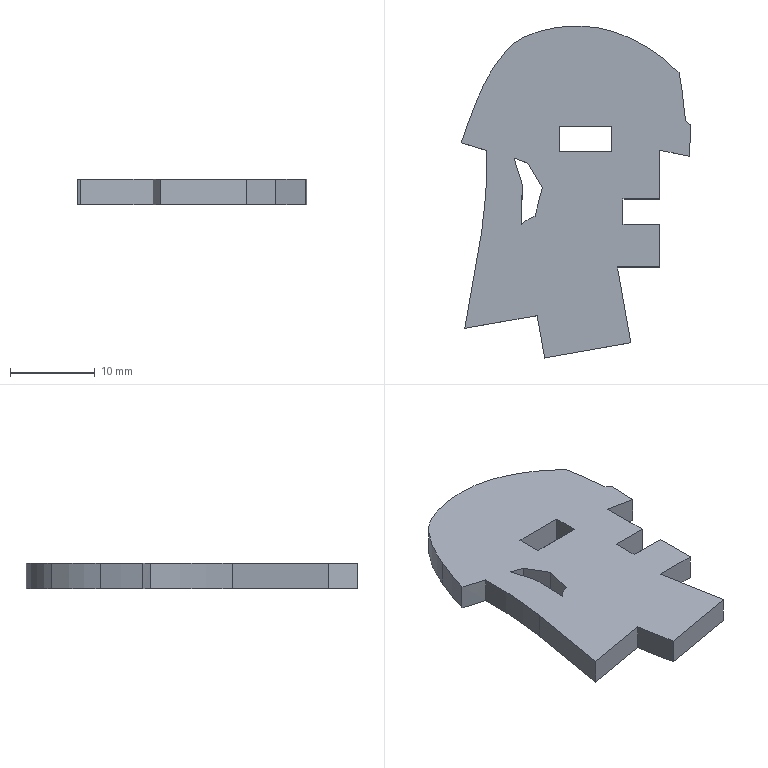Part | SolidWorks | features BaseBody 1 | 1 solid | 33 faces | box 27.077 x 39.16 x 3 mm | volume 2127 mm3 | plane 20 | spline 13
STEP:
#1=CARTESIAN_POINT('',(-12.743,15.285,-1.5));
#2=VERTEX_POINT('',#1);
#3=CARTESIAN_POINT('',(-6.608,15.285,-1.5));
#4=VERTEX_POINT('',#3);
#5=CARTESIAN_POINT('',(-12.743,15.285,-1.5));
#6=DIRECTION('',(1.,0.,0.));
#7=VECTOR('',#6,1000.);
#8=LINE('',#5,#7);
#9=EDGE_CURVE('',#2,#4,#8,.T.);
#10=ORIENTED_EDGE('',*,*,#9,.F.);
#11=CARTESIAN_POINT('',(-12.743,15.285,1.5));
#12=VERTEX_POINT('',#11);
#13=CARTESIAN_POINT('',(-12.743,15.285,1.5));
#14=DIRECTION('',(0.,0.,-1.));
#15=VECTOR('',#14,1000.);
#16=LINE('',#13,#15);
#17=EDGE_CURVE('',#12,#2,#16,.T.);
#18=ORIENTED_EDGE('',*,*,#17,.F.);
#19=CARTESIAN_POINT('',(-6.608,15.285,1.5));
#20=VERTEX_POINT('',#19);
#21=CARTESIAN_POINT('',(-12.743,15.285,1.5));
#22=DIRECTION('',(1.,0.,0.));
#23=VECTOR('',#22,1000.);
#24=LINE('',#21,#23);
#25=EDGE_CURVE('',#12,#20,#24,.T.);
#26=ORIENTED_EDGE('',*,*,#25,.T.);
#27=CARTESIAN_POINT('',(-6.608,15.285,1.5));
#28=DIRECTION('',(0.,0.,-1.));
#29=VECTOR('',#28,1000.);
#30=LINE('',#27,#29);
#31=EDGE_CURVE('',#20,#4,#30,.T.);
#32=ORIENTED_EDGE('',*,*,#31,.T.);
#33=EDGE_LOOP('',(#10,#18,#26,#32));
#34=FACE_OUTER_BOUND('',#33,.T.);
#35=CARTESIAN_POINT('',(-12.743,15.285,1.5));
#36=DIRECTION('',(0.,1.,0.));
#37=DIRECTION('',(1.,0.,0.));
#38=AXIS2_PLACEMENT_3D('',#35,#36,#37);
#39=PLANE('',#38);
#40=ADVANCED_FACE('',(#34),#39,.T.);
#41=CARTESIAN_POINT('',(-12.743,18.281,-1.5));
#42=VERTEX_POINT('',#41);
#43=CARTESIAN_POINT('',(-12.743,18.281,-1.5));
#44=DIRECTION('',(0.,-1.,0.));
#45=VECTOR('',#44,1000.);
#46=LINE('',#43,#45);
#47=EDGE_CURVE('',#42,#2,#46,.T.);
#48=ORIENTED_EDGE('',*,*,#47,.F.);
#49=CARTESIAN_POINT('',(-12.743,18.281,1.5));
#50=VERTEX_POINT('',#49);
#51=CARTESIAN_POINT('',(-12.743,18.281,1.5));
#52=DIRECTION('',(0.,0.,-1.));
#53=VECTOR('',#52,1000.);
#54=LINE('',#51,#53);
#55=EDGE_CURVE('',#50,#42,#54,.T.);
#56=ORIENTED_EDGE('',*,*,#55,.F.);
#57=CARTESIAN_POINT('',(-12.743,18.281,1.5));
#58=DIRECTION('',(0.,-1.,0.));
#59=VECTOR('',#58,1000.);
#60=LINE('',#57,#59);
#61=EDGE_CURVE('',#50,#12,#60,.T.);
#62=ORIENTED_EDGE('',*,*,#61,.T.);
#63=ORIENTED_EDGE('',*,*,#17,.T.);
#64=EDGE_LOOP('',(#48,#56,#62,#63));
#65=FACE_OUTER_BOUND('',#64,.T.);
#66=CARTESIAN_POINT('',(-12.743,18.281,1.5));
#67=DIRECTION('',(1.,0.,0.));
#68=DIRECTION('',(0.,1.,0.));
#69=AXIS2_PLACEMENT_3D('',#66,#67,#68);
#70=PLANE('',#69);
#71=ADVANCED_FACE('',(#65),#70,.T.);
#72=CARTESIAN_POINT('',(-6.608,18.281,-1.5));
#73=VERTEX_POINT('',#72);
#74=CARTESIAN_POINT('',(-6.608,18.281,-1.5));
#75=DIRECTION('',(-1.,0.,0.));
#76=VECTOR('',#75,1000.);
#77=LINE('',#74,#76);
#78=EDGE_CURVE('',#73,#42,#77,.T.);
#79=ORIENTED_EDGE('',*,*,#78,.F.);
#80=CARTESIAN_POINT('',(-6.608,18.281,1.5));
#81=VERTEX_POINT('',#80);
#82=CARTESIAN_POINT('',(-6.608,18.281,1.5));
#83=DIRECTION('',(0.,0.,-1.));
#84=VECTOR('',#83,1000.);
#85=LINE('',#82,#84);
#86=EDGE_CURVE('',#81,#73,#85,.T.);
#87=ORIENTED_EDGE('',*,*,#86,.F.);
#88=CARTESIAN_POINT('',(-6.608,18.281,1.5));
#89=DIRECTION('',(-1.,0.,0.));
#90=VECTOR('',#89,1000.);
#91=LINE('',#88,#90);
#92=EDGE_CURVE('',#81,#50,#91,.T.);
#93=ORIENTED_EDGE('',*,*,#92,.T.);
#94=ORIENTED_EDGE('',*,*,#55,.T.);
#95=EDGE_LOOP('',(#79,#87,#93,#94));
#96=FACE_OUTER_BOUND('',#95,.T.);
#97=CARTESIAN_POINT('',(-6.608,18.281,1.5));
#98=DIRECTION('',(0.,-1.,0.));
#99=DIRECTION('',(0.,0.,-1.));
#100=AXIS2_PLACEMENT_3D('',#97,#98,#99);
#101=PLANE('',#100);
#102=ADVANCED_FACE('',(#96),#101,.T.);
#103=CARTESIAN_POINT('',(-6.608,15.285,-1.5));
#104=DIRECTION('',(0.,1.,0.));
#105=VECTOR('',#104,1000.);
#106=LINE('',#103,#105);
#107=EDGE_CURVE('',#4,#73,#106,.T.);
#108=ORIENTED_EDGE('',*,*,#107,.F.);
#109=ORIENTED_EDGE('',*,*,#31,.F.);
#110=CARTESIAN_POINT('',(-6.608,15.285,1.5));
#111=DIRECTION('',(0.,1.,0.));
#112=VECTOR('',#111,1000.);
#113=LINE('',#110,#112);
#114=EDGE_CURVE('',#20,#81,#113,.T.);
#115=ORIENTED_EDGE('',*,*,#114,.T.);
#116=ORIENTED_EDGE('',*,*,#86,.T.);
#117=EDGE_LOOP('',(#108,#109,#115,#116));
#118=FACE_OUTER_BOUND('',#117,.T.);
#119=CARTESIAN_POINT('',(-6.608,15.285,1.5));
#120=DIRECTION('',(-1.,0.,0.));
#121=DIRECTION('',(0.,1.,0.));
#122=AXIS2_PLACEMENT_3D('',#119,#120,#121);
#123=PLANE('',#122);
#124=ADVANCED_FACE('',(#118),#123,.T.);
#125=CARTESIAN_POINT('',(-16.5,13.932,-1.5));
#126=VERTEX_POINT('',#125);
#127=CARTESIAN_POINT('',(-18.124,14.526,-1.5));
#128=VERTEX_POINT('',#127);
#129=CARTESIAN_POINT('',(-16.5,13.932,-1.5));
#130=CARTESIAN_POINT('',(-17.041,14.129,-1.5));
#131=CARTESIAN_POINT('',(-17.583,14.328,-1.5));
#132=CARTESIAN_POINT('',(-18.124,14.526,-1.5));
#133=B_SPLINE_CURVE_WITH_KNOTS('',3,(#129,#130,#131,#132),.UNSPECIFIED.,.F.,.F.,(4,4),(0.,0.1429),.UNSPECIFIED.);
#134=EDGE_CURVE('',#126,#128,#133,.T.);
#135=ORIENTED_EDGE('',*,*,#134,.F.);
#136=CARTESIAN_POINT('',(-16.5,13.932,1.5));
#137=VERTEX_POINT('',#136);
#138=CARTESIAN_POINT('',(-16.5,13.932,1.5));
#139=DIRECTION('',(0.,0.,-1.));
#140=VECTOR('',#139,1000.);
#141=LINE('',#138,#140);
#142=EDGE_CURVE('',#137,#126,#141,.T.);
#143=ORIENTED_EDGE('',*,*,#142,.F.);
#144=CARTESIAN_POINT('',(-18.124,14.526,1.5));
#145=VERTEX_POINT('',#144);
#146=CARTESIAN_POINT('',(-16.5,13.932,1.5));
#147=CARTESIAN_POINT('',(-17.041,14.129,1.5));
#148=CARTESIAN_POINT('',(-17.583,14.328,1.5));
#149=CARTESIAN_POINT('',(-18.124,14.526,1.5));
#150=B_SPLINE_CURVE_WITH_KNOTS('',3,(#146,#147,#148,#149),.UNSPECIFIED.,.F.,.F.,(4,4),(0.,0.1429),.UNSPECIFIED.);
#151=EDGE_CURVE('',#137,#145,#150,.T.);
#152=ORIENTED_EDGE('',*,*,#151,.T.);
#153=CARTESIAN_POINT('',(-18.124,14.526,1.5));
#154=DIRECTION('',(0.,0.,-1.));
#155=VECTOR('',#154,1000.);
#156=LINE('',#153,#155);
#157=EDGE_CURVE('',#145,#128,#156,.T.);
#158=ORIENTED_EDGE('',*,*,#157,.T.);
#159=EDGE_LOOP('',(#135,#143,#152,#158));
#160=FACE_OUTER_BOUND('',#159,.T.);
#161=CARTESIAN_POINT('',(-16.5,13.932,1.5));
#162=CARTESIAN_POINT('',(-16.5,13.932,-1.5));
#163=CARTESIAN_POINT('',(-17.041,14.129,1.5));
#164=CARTESIAN_POINT('',(-17.041,14.129,-1.5));
#165=CARTESIAN_POINT('',(-17.583,14.328,1.5));
#166=CARTESIAN_POINT('',(-17.583,14.328,-1.5));
#167=CARTESIAN_POINT('',(-18.124,14.526,1.5));
#168=CARTESIAN_POINT('',(-18.124,14.526,-1.5));
#169=B_SPLINE_SURFACE_WITH_KNOTS('',3,1,((#161,#162),(#163,#164),(#165,#166),(#167,#168)),.UNSPECIFIED.,.F.,.F.,.F.,(4,4),(2,2),(0.,0.1429),(0.,1.),.UNSPECIFIED.);
#170=ADVANCED_FACE('',(#160),#169,.T.);
#171=CARTESIAN_POINT('',(-14.796,11.064,-1.5));
#172=VERTEX_POINT('',#171);
#173=CARTESIAN_POINT('',(-14.796,11.064,-1.5));
#174=CARTESIAN_POINT('',(-15.362,12.021,-1.5));
#175=CARTESIAN_POINT('',(-15.932,12.975,-1.5));
#176=CARTESIAN_POINT('',(-16.5,13.932,-1.5));
#177=B_SPLINE_CURVE_WITH_KNOTS('',3,(#173,#174,#175,#176),.UNSPECIFIED.,.F.,.F.,(4,4),(0.1429,0.2857),.UNSPECIFIED.);
#178=EDGE_CURVE('',#172,#126,#177,.T.);
#179=ORIENTED_EDGE('',*,*,#178,.F.);
#180=CARTESIAN_POINT('',(-14.796,11.064,1.5));
#181=VERTEX_POINT('',#180);
#182=CARTESIAN_POINT('',(-14.796,11.064,1.5));
#183=DIRECTION('',(0.,0.,-1.));
#184=VECTOR('',#183,1000.);
#185=LINE('',#182,#184);
#186=EDGE_CURVE('',#181,#172,#185,.T.);
#187=ORIENTED_EDGE('',*,*,#186,.F.);
#188=CARTESIAN_POINT('',(-14.796,11.064,1.5));
#189=CARTESIAN_POINT('',(-15.362,12.021,1.5));
#190=CARTESIAN_POINT('',(-15.932,12.975,1.5));
#191=CARTESIAN_POINT('',(-16.5,13.932,1.5));
#192=B_SPLINE_CURVE_WITH_KNOTS('',3,(#188,#189,#190,#191),.UNSPECIFIED.,.F.,.F.,(4,4),(0.1429,0.2857),.UNSPECIFIED.);
#193=EDGE_CURVE('',#181,#137,#192,.T.);
#194=ORIENTED_EDGE('',*,*,#193,.T.);
#195=ORIENTED_EDGE('',*,*,#142,.T.);
#196=EDGE_LOOP('',(#179,#187,#194,#195));
#197=FACE_OUTER_BOUND('',#196,.T.);
#198=CARTESIAN_POINT('',(-14.796,11.064,1.5));
#199=CARTESIAN_POINT('',(-14.796,11.064,-1.5));
#200=CARTESIAN_POINT('',(-15.362,12.021,1.5));
#201=CARTESIAN_POINT('',(-15.362,12.021,-1.5));
#202=CARTESIAN_POINT('',(-15.932,12.975,1.5));
#203=CARTESIAN_POINT('',(-15.932,12.975,-1.5));
#204=CARTESIAN_POINT('',(-16.5,13.932,1.5));
#205=CARTESIAN_POINT('',(-16.5,13.932,-1.5));
#206=B_SPLINE_SURFACE_WITH_KNOTS('',3,1,((#198,#199),(#200,#201),(#202,#203),(#204,#205)),.UNSPECIFIED.,.F.,.F.,.F.,(4,4),(2,2),(0.1429,0.2857),(0.,1.),.UNSPECIFIED.);
#207=ADVANCED_FACE('',(#197),#206,.T.);
#208=CARTESIAN_POINT('',(-15.657,7.675,-1.5));
#209=VERTEX_POINT('',#208);
#210=CARTESIAN_POINT('',(-15.657,7.675,-1.5));
#211=CARTESIAN_POINT('',(-15.369,8.805,-1.5));
#212=CARTESIAN_POINT('',(-15.081,9.935,-1.5));
#213=CARTESIAN_POINT('',(-14.796,11.064,-1.5));
#214=B_SPLINE_CURVE_WITH_KNOTS('',3,(#210,#211,#212,#213),.UNSPECIFIED.,.F.,.F.,(4,4),(0.2857,0.4286),.UNSPECIFIED.);
#215=EDGE_CURVE('',#209,#172,#214,.T.);
#216=ORIENTED_EDGE('',*,*,#215,.F.);
#217=CARTESIAN_POINT('',(-15.657,7.675,1.5));
#218=VERTEX_POINT('',#217);
#219=CARTESIAN_POINT('',(-15.657,7.675,1.5));
#220=DIRECTION('',(0.,0.,-1.));
#221=VECTOR('',#220,1000.);
#222=LINE('',#219,#221);
#223=EDGE_CURVE('',#218,#209,#222,.T.);
#224=ORIENTED_EDGE('',*,*,#223,.F.);
#225=CARTESIAN_POINT('',(-15.657,7.675,1.5));
#226=CARTESIAN_POINT('',(-15.369,8.805,1.5));
#227=CARTESIAN_POINT('',(-15.081,9.935,1.5));
#228=CARTESIAN_POINT('',(-14.796,11.064,1.5));
#229=B_SPLINE_CURVE_WITH_KNOTS('',3,(#225,#226,#227,#228),.UNSPECIFIED.,.F.,.F.,(4,4),(0.2857,0.4286),.UNSPECIFIED.);
#230=EDGE_CURVE('',#218,#181,#229,.T.);
#231=ORIENTED_EDGE('',*,*,#230,.T.);
#232=ORIENTED_EDGE('',*,*,#186,.T.);
#233=EDGE_LOOP('',(#216,#224,#231,#232));
#234=FACE_OUTER_BOUND('',#233,.T.);
#235=CARTESIAN_POINT('',(-15.657,7.675,1.5));
#236=CARTESIAN_POINT('',(-15.657,7.675,-1.5));
#237=CARTESIAN_POINT('',(-15.369,8.805,1.5));
#238=CARTESIAN_POINT('',(-15.369,8.805,-1.5));
#239=CARTESIAN_POINT('',(-15.081,9.935,1.5));
#240=CARTESIAN_POINT('',(-15.081,9.935,-1.5));
#241=CARTESIAN_POINT('',(-14.796,11.064,1.5));
#242=CARTESIAN_POINT('',(-14.796,11.064,-1.5));
#243=B_SPLINE_SURFACE_WITH_KNOTS('',3,1,((#235,#236),(#237,#238),(#239,#240),(#241,#242)),.UNSPECIFIED.,.F.,.F.,.F.,(4,4),(2,2),(0.2857,0.4286),(0.,1.),.UNSPECIFIED.);
#244=ADVANCED_FACE('',(#234),#243,.T.);
#245=CARTESIAN_POINT('',(-17.304,6.657,-1.5));
#246=VERTEX_POINT('',#245);
#247=CARTESIAN_POINT('',(-17.304,6.657,-1.5));
#248=CARTESIAN_POINT('',(-16.762,7.199,-1.5));
#249=CARTESIAN_POINT('',(-16.21,7.436,-1.5));
#250=CARTESIAN_POINT('',(-15.657,7.675,-1.5));
#251=B_SPLINE_CURVE_WITH_KNOTS('',3,(#247,#248,#249,#250),.UNSPECIFIED.,.F.,.F.,(4,4),(0.4286,0.5714),.UNSPECIFIED.);
#252=EDGE_CURVE('',#246,#209,#251,.T.);
#253=ORIENTED_EDGE('',*,*,#252,.F.);
#254=CARTESIAN_POINT('',(-17.304,6.657,1.5));
#255=VERTEX_POINT('',#254);
#256=CARTESIAN_POINT('',(-17.304,6.657,1.5));
#257=DIRECTION('',(0.,0.,-1.));
#258=VECTOR('',#257,1000.);
#259=LINE('',#256,#258);
#260=EDGE_CURVE('',#255,#246,#259,.T.);
#261=ORIENTED_EDGE('',*,*,#260,.F.);
#262=CARTESIAN_POINT('',(-17.304,6.657,1.5));
#263=CARTESIAN_POINT('',(-16.762,7.199,1.5));
#264=CARTESIAN_POINT('',(-16.21,7.436,1.5));
#265=CARTESIAN_POINT('',(-15.657,7.675,1.5));
#266=B_SPLINE_CURVE_WITH_KNOTS('',3,(#262,#263,#264,#265),.UNSPECIFIED.,.F.,.F.,(4,4),(0.4286,0.5714),.UNSPECIFIED.);
#267=EDGE_CURVE('',#255,#218,#266,.T.);
#268=ORIENTED_EDGE('',*,*,#267,.T.);
#269=ORIENTED_EDGE('',*,*,#223,.T.);
#270=EDGE_LOOP('',(#253,#261,#268,#269));
#271=FACE_OUTER_BOUND('',#270,.T.);
#272=CARTESIAN_POINT('',(-17.304,6.657,1.5));
#273=CARTESIAN_POINT('',(-17.304,6.657,-1.5));
#274=CARTESIAN_POINT('',(-16.762,7.199,1.5));
#275=CARTESIAN_POINT('',(-16.762,7.199,-1.5));
#276=CARTESIAN_POINT('',(-16.21,7.436,1.5));
#277=CARTESIAN_POINT('',(-16.21,7.436,-1.5));
#278=CARTESIAN_POINT('',(-15.657,7.675,1.5));
#279=CARTESIAN_POINT('',(-15.657,7.675,-1.5));
#280=B_SPLINE_SURFACE_WITH_KNOTS('',3,1,((#272,#273),(#274,#275),(#276,#277),(#278,#279)),.UNSPECIFIED.,.F.,.F.,.F.,(4,4),(2,2),(0.4286,0.5714),(0.,1.),.UNSPECIFIED.);
#281=ADVANCED_FACE('',(#271),#280,.T.);
#282=CARTESIAN_POINT('',(-17.159,11.364,-1.5));
#283=VERTEX_POINT('',#282);
#284=CARTESIAN_POINT('',(-17.159,11.364,-1.5));
#285=CARTESIAN_POINT('',(-17.195,9.226,-1.5));
#286=CARTESIAN_POINT('',(-17.232,7.091,-1.5));
#287=CARTESIAN_POINT('',(-17.304,6.657,-1.5));
#288=B_SPLINE_CURVE_WITH_KNOTS('',3,(#284,#285,#286,#287),.UNSPECIFIED.,.F.,.F.,(4,4),(0.5714,0.7143),.UNSPECIFIED.);
#289=EDGE_CURVE('',#283,#246,#288,.T.);
#290=ORIENTED_EDGE('',*,*,#289,.F.);
#291=CARTESIAN_POINT('',(-17.159,11.364,1.5));
#292=VERTEX_POINT('',#291);
#293=CARTESIAN_POINT('',(-17.159,11.364,1.5));
#294=DIRECTION('',(0.,0.,-1.));
#295=VECTOR('',#294,1000.);
#296=LINE('',#293,#295);
#297=EDGE_CURVE('',#292,#283,#296,.T.);
#298=ORIENTED_EDGE('',*,*,#297,.F.);
#299=CARTESIAN_POINT('',(-17.159,11.364,1.5));
#300=CARTESIAN_POINT('',(-17.195,9.226,1.5));
#301=CARTESIAN_POINT('',(-17.232,7.091,1.5));
#302=CARTESIAN_POINT('',(-17.304,6.657,1.5));
#303=B_SPLINE_CURVE_WITH_KNOTS('',3,(#299,#300,#301,#302),.UNSPECIFIED.,.F.,.F.,(4,4),(0.5714,0.7143),.UNSPECIFIED.);
#304=EDGE_CURVE('',#292,#255,#303,.T.);
#305=ORIENTED_EDGE('',*,*,#304,.T.);
#306=ORIENTED_EDGE('',*,*,#260,.T.);
#307=EDGE_LOOP('',(#290,#298,#305,#306));
#308=FACE_OUTER_BOUND('',#307,.T.);
#309=CARTESIAN_POINT('',(-17.159,11.364,1.5));
#310=CARTESIAN_POINT('',(-17.159,11.364,-1.5));
#311=CARTESIAN_POINT('',(-17.195,9.226,1.5));
#312=CARTESIAN_POINT('',(-17.195,9.226,-1.5));
#313=CARTESIAN_POINT('',(-17.232,7.091,1.5));
#314=CARTESIAN_POINT('',(-17.232,7.091,-1.5));
#315=CARTESIAN_POINT('',(-17.304,6.657,1.5));
#316=CARTESIAN_POINT('',(-17.304,6.657,-1.5));
#317=B_SPLINE_SURFACE_WITH_KNOTS('',3,1,((#309,#310),(#311,#312),(#313,#314),(#315,#316)),.UNSPECIFIED.,.F.,.F.,.F.,(4,4),(2,2),(0.5714,0.7143),(0.,1.),.UNSPECIFIED.);
#318=ADVANCED_FACE('',(#308),#317,.T.);
#319=CARTESIAN_POINT('',(-18.124,14.526,-1.5));
#320=CARTESIAN_POINT('',(-17.802,13.472,-1.5));
#321=CARTESIAN_POINT('',(-17.481,12.418,-1.5));
#322=CARTESIAN_POINT('',(-17.159,11.364,-1.5));
#323=B_SPLINE_CURVE_WITH_KNOTS('',3,(#319,#320,#321,#322),.UNSPECIFIED.,.F.,.F.,(4,4),(0.7143,1.),.UNSPECIFIED.);
#324=EDGE_CURVE('',#128,#283,#323,.T.);
#325=ORIENTED_EDGE('',*,*,#324,.F.);
#326=ORIENTED_EDGE('',*,*,#157,.F.);
#327=CARTESIAN_POINT('',(-18.124,14.526,1.5));
#328=CARTESIAN_POINT('',(-17.802,13.472,1.5));
#329=CARTESIAN_POINT('',(-17.481,12.418,1.5));
#330=CARTESIAN_POINT('',(-17.159,11.364,1.5));
#331=B_SPLINE_CURVE_WITH_KNOTS('',3,(#327,#328,#329,#330),.UNSPECIFIED.,.F.,.F.,(4,4),(0.7143,1.),.UNSPECIFIED.);
#332=EDGE_CURVE('',#145,#292,#331,.T.);
#333=ORIENTED_EDGE('',*,*,#332,.T.);
#334=ORIENTED_EDGE('',*,*,#297,.T.);
#335=EDGE_LOOP('',(#325,#326,#333,#334));
#336=FACE_OUTER_BOUND('',#335,.T.);
#337=CARTESIAN_POINT('',(-18.124,14.526,1.5));
#338=CARTESIAN_POINT('',(-18.124,14.526,-1.5));
#339=CARTESIAN_POINT('',(-17.802,13.472,1.5));
#340=CARTESIAN_POINT('',(-17.802,13.472,-1.5));
#341=CARTESIAN_POINT('',(-17.481,12.418,1.5));
#342=CARTESIAN_POINT('',(-17.481,12.418,-1.5));
#343=CARTESIAN_POINT('',(-17.159,11.364,1.5));
#344=CARTESIAN_POINT('',(-17.159,11.364,-1.5));
#345=B_SPLINE_SURFACE_WITH_KNOTS('',3,1,((#337,#338),(#339,#340),(#341,#342),(#343,#344)),.UNSPECIFIED.,.F.,.F.,.F.,(4,4),(2,2),(0.7143,1.),(0.,1.),.UNSPECIFIED.);
#346=ADVANCED_FACE('',(#336),#345,.T.);
#347=CARTESIAN_POINT('',(-21.328,15.424,-1.5));
#348=VERTEX_POINT('',#347);
#349=CARTESIAN_POINT('',(-21.967,5.773,-1.5));
#350=VERTEX_POINT('',#349);
#351=CARTESIAN_POINT('',(-21.328,15.424,-1.5));
#352=CARTESIAN_POINT('',(-21.217,11.828,-1.5));
#353=CARTESIAN_POINT('',(-21.591,8.801,-1.5));
#354=CARTESIAN_POINT('',(-21.967,5.773,-1.5));
#355=B_SPLINE_CURVE_WITH_KNOTS('',3,(#351,#352,#353,#354),.UNSPECIFIED.,.F.,.F.,(4,4),(0.06879,0.1033),.UNSPECIFIED.);
#356=EDGE_CURVE('',#348,#350,#355,.T.);
#357=ORIENTED_EDGE('',*,*,#356,.T.);
#358=CARTESIAN_POINT('',(-21.967,5.773,1.5));
#359=VERTEX_POINT('',#358);
#360=CARTESIAN_POINT('',(-21.967,5.773,1.5));
#361=DIRECTION('',(0.,0.,-1.));
#362=VECTOR('',#361,1000.);
#363=LINE('',#360,#362);
#364=EDGE_CURVE('',#359,#350,#363,.T.);
#365=ORIENTED_EDGE('',*,*,#364,.F.);
#366=CARTESIAN_POINT('',(-21.328,15.424,1.5));
#367=VERTEX_POINT('',#366);
#368=CARTESIAN_POINT('',(-21.328,15.424,1.5));
#369=CARTESIAN_POINT('',(-21.217,11.828,1.5));
#370=CARTESIAN_POINT('',(-21.591,8.801,1.5));
#371=CARTESIAN_POINT('',(-21.967,5.773,1.5));
#372=B_SPLINE_CURVE_WITH_KNOTS('',3,(#368,#369,#370,#371),.UNSPECIFIED.,.F.,.F.,(4,4),(0.06879,0.1033),.UNSPECIFIED.);
#373=EDGE_CURVE('',#367,#359,#372,.T.);
#374=ORIENTED_EDGE('',*,*,#373,.F.);
#375=CARTESIAN_POINT('',(-21.328,15.424,1.5));
#376=DIRECTION('',(0.,0.,-1.));
#377=VECTOR('',#376,1000.);
#378=LINE('',#375,#377);
#379=EDGE_CURVE('',#367,#348,#378,.T.);
#380=ORIENTED_EDGE('',*,*,#379,.T.);
#381=EDGE_LOOP('',(#357,#365,#374,#380));
#382=FACE_OUTER_BOUND('',#381,.T.);
#383=CARTESIAN_POINT('',(-21.328,15.424,1.5));
#384=CARTESIAN_POINT('',(-21.328,15.424,-1.5));
#385=CARTESIAN_POINT('',(-21.217,11.828,1.5));
#386=CARTESIAN_POINT('',(-21.217,11.828,-1.5));
#387=CARTESIAN_POINT('',(-21.591,8.801,1.5));
#388=CARTESIAN_POINT('',(-21.591,8.801,-1.5));
#389=CARTESIAN_POINT('',(-21.967,5.773,1.5));
#390=CARTESIAN_POINT('',(-21.967,5.773,-1.5));
#391=B_SPLINE_SURFACE_WITH_KNOTS('',3,1,((#383,#384),(#385,#386),(#387,#388),(#389,#390)),.UNSPECIFIED.,.F.,.F.,.F.,(4,4),(2,2),(0.06879,0.1033),(0.,1.),.UNSPECIFIED.);
#392=ADVANCED_FACE('',(#382),#391,.F.);
#393=CARTESIAN_POINT('',(-24.361,16.333,-1.5));
#394=VERTEX_POINT('',#393);
#395=CARTESIAN_POINT('',(-24.361,16.333,-1.5));
#396=CARTESIAN_POINT('',(-23.199,15.969,-1.5));
#397=CARTESIAN_POINT('',(-22.033,15.607,-1.5));
#398=CARTESIAN_POINT('',(-21.328,15.424,-1.5));
#399=B_SPLINE_CURVE_WITH_KNOTS('',3,(#395,#396,#397,#398),.UNSPECIFIED.,.F.,.F.,(4,4),(0.1033,0.1378),.UNSPECIFIED.);
#400=EDGE_CURVE('',#394,#348,#399,.T.);
#401=ORIENTED_EDGE('',*,*,#400,.T.);
#402=ORIENTED_EDGE('',*,*,#379,.F.);
#403=CARTESIAN_POINT('',(-24.361,16.333,1.5));
#404=VERTEX_POINT('',#403);
#405=CARTESIAN_POINT('',(-24.361,16.333,1.5));
#406=CARTESIAN_POINT('',(-23.199,15.969,1.5));
#407=CARTESIAN_POINT('',(-22.033,15.607,1.5));
#408=CARTESIAN_POINT('',(-21.328,15.424,1.5));
#409=B_SPLINE_CURVE_WITH_KNOTS('',3,(#405,#406,#407,#408),.UNSPECIFIED.,.F.,.F.,(4,4),(0.1033,0.1378),.UNSPECIFIED.);
#410=EDGE_CURVE('',#404,#367,#409,.T.);
#411=ORIENTED_EDGE('',*,*,#410,.F.);
#412=CARTESIAN_POINT('',(-24.361,16.333,1.5));
#413=DIRECTION('',(0.,0.,-1.));
#414=VECTOR('',#413,1000.);
#415=LINE('',#412,#414);
#416=EDGE_CURVE('',#404,#394,#415,.T.);
#417=ORIENTED_EDGE('',*,*,#416,.T.);
#418=EDGE_LOOP('',(#401,#402,#411,#417));
#419=FACE_OUTER_BOUND('',#418,.T.);
#420=CARTESIAN_POINT('',(-24.361,16.333,1.5));
#421=CARTESIAN_POINT('',(-24.361,16.333,-1.5));
#422=CARTESIAN_POINT('',(-23.199,15.969,1.5));
#423=CARTESIAN_POINT('',(-23.199,15.969,-1.5));
#424=CARTESIAN_POINT('',(-22.033,15.607,1.5));
#425=CARTESIAN_POINT('',(-22.033,15.607,-1.5));
#426=CARTESIAN_POINT('',(-21.328,15.424,1.5));
#427=CARTESIAN_POINT('',(-21.328,15.424,-1.5));
#428=B_SPLINE_SURFACE_WITH_KNOTS('',3,1,((#420,#421),(#422,#423),(#424,#425),(#426,#427)),.UNSPECIFIED.,.F.,.F.,.F.,(4,4),(2,2),(0.1033,0.1378),(0.,1.),.UNSPECIFIED.);
#429=ADVANCED_FACE('',(#419),#428,.F.);
#430=CARTESIAN_POINT('',(-22.511,21.351,-1.5));
#431=VERTEX_POINT('',#430);
#432=CARTESIAN_POINT('',(-22.511,21.351,-1.5));
#433=CARTESIAN_POINT('',(-23.452,19.062,-1.5));
#434=CARTESIAN_POINT('',(-23.907,17.697,-1.5));
#435=CARTESIAN_POINT('',(-24.361,16.333,-1.5));
#436=B_SPLINE_CURVE_WITH_KNOTS('',3,(#432,#433,#434,#435),.UNSPECIFIED.,.F.,.F.,(4,4),(0.1378,0.1722),.UNSPECIFIED.);
#437=EDGE_CURVE('',#431,#394,#436,.T.);
#438=ORIENTED_EDGE('',*,*,#437,.T.);
#439=ORIENTED_EDGE('',*,*,#416,.F.);
#440=CARTESIAN_POINT('',(-22.511,21.351,1.5));
#441=VERTEX_POINT('',#440);
#442=CARTESIAN_POINT('',(-22.511,21.351,1.5));
#443=CARTESIAN_POINT('',(-23.452,19.062,1.5));
#444=CARTESIAN_POINT('',(-23.907,17.697,1.5));
#445=CARTESIAN_POINT('',(-24.361,16.333,1.5));
#446=B_SPLINE_CURVE_WITH_KNOTS('',3,(#442,#443,#444,#445),.UNSPECIFIED.,.F.,.F.,(4,4),(0.1378,0.1722),.UNSPECIFIED.);
#447=EDGE_CURVE('',#441,#404,#446,.T.);
#448=ORIENTED_EDGE('',*,*,#447,.F.);
#449=CARTESIAN_POINT('',(-22.511,21.351,1.5));
#450=DIRECTION('',(0.,0.,-1.));
#451=VECTOR('',#450,1000.);
#452=LINE('',#449,#451);
#453=EDGE_CURVE('',#441,#431,#452,.T.);
#454=ORIENTED_EDGE('',*,*,#453,.T.);
#455=EDGE_LOOP('',(#438,#439,#448,#454));
#456=FACE_OUTER_BOUND('',#455,.T.);
#457=CARTESIAN_POINT('',(-22.511,21.351,1.5));
#458=CARTESIAN_POINT('',(-22.511,21.351,-1.5));
#459=CARTESIAN_POINT('',(-23.452,19.062,1.5));
#460=CARTESIAN_POINT('',(-23.452,19.062,-1.5));
#461=CARTESIAN_POINT('',(-23.907,17.697,1.5));
#462=CARTESIAN_POINT('',(-23.907,17.697,-1.5));
#463=CARTESIAN_POINT('',(-24.361,16.333,1.5));
#464=CARTESIAN_POINT('',(-24.361,16.333,-1.5));
#465=B_SPLINE_SURFACE_WITH_KNOTS('',3,1,((#457,#458),(#459,#460),(#461,#462),(#463,#464)),.UNSPECIFIED.,.F.,.F.,.F.,(4,4),(2,2),(0.1378,0.1722),(0.,1.),.UNSPECIFIED.);
#466=ADVANCED_FACE('',(#456),#465,.F.);
#467=CARTESIAN_POINT('',(-19.129,27.113,-1.5));
#468=VERTEX_POINT('',#467);
#469=CARTESIAN_POINT('',(-19.129,27.113,-1.5));
#470=CARTESIAN_POINT('',(-21.019,24.847,-1.5));
#471=CARTESIAN_POINT('',(-21.691,23.345,-1.5));
#472=CARTESIAN_POINT('',(-22.511,21.351,-1.5));
#473=B_SPLINE_CURVE_WITH_KNOTS('',3,(#469,#470,#471,#472),.UNSPECIFIED.,.F.,.F.,(4,4),(0.1722,0.2067),.UNSPECIFIED.);
#474=EDGE_CURVE('',#468,#431,#473,.T.);
#475=ORIENTED_EDGE('',*,*,#474,.T.);
#476=ORIENTED_EDGE('',*,*,#453,.F.);
#477=CARTESIAN_POINT('',(-19.129,27.113,1.5));
#478=VERTEX_POINT('',#477);
#479=CARTESIAN_POINT('',(-19.129,27.113,1.5));
#480=CARTESIAN_POINT('',(-21.019,24.847,1.5));
#481=CARTESIAN_POINT('',(-21.691,23.345,1.5));
#482=CARTESIAN_POINT('',(-22.511,21.351,1.5));
#483=B_SPLINE_CURVE_WITH_KNOTS('',3,(#479,#480,#481,#482),.UNSPECIFIED.,.F.,.F.,(4,4),(0.1722,0.2067),.UNSPECIFIED.);
#484=EDGE_CURVE('',#478,#441,#483,.T.);
#485=ORIENTED_EDGE('',*,*,#484,.F.);
#486=CARTESIAN_POINT('',(-19.129,27.113,1.5));
#487=DIRECTION('',(0.,0.,-1.));
#488=VECTOR('',#487,1000.);
#489=LINE('',#486,#488);
#490=EDGE_CURVE('',#478,#468,#489,.T.);
#491=ORIENTED_EDGE('',*,*,#490,.T.);
#492=EDGE_LOOP('',(#475,#476,#485,#491));
#493=FACE_OUTER_BOUND('',#492,.T.);
#494=CARTESIAN_POINT('',(-19.129,27.113,1.5));
#495=CARTESIAN_POINT('',(-19.129,27.113,-1.5));
#496=CARTESIAN_POINT('',(-21.019,24.847,1.5));
#497=CARTESIAN_POINT('',(-21.019,24.847,-1.5));
#498=CARTESIAN_POINT('',(-21.691,23.345,1.5));
#499=CARTESIAN_POINT('',(-21.691,23.345,-1.5));
#500=CARTESIAN_POINT('',(-22.511,21.351,1.5));
#501=CARTESIAN_POINT('',(-22.511,21.351,-1.5));
#502=B_SPLINE_SURFACE_WITH_KNOTS('',3,1,((#494,#495),(#496,#497),(#498,#499),(#500,#501)),.UNSPECIFIED.,.F.,.F.,.F.,(4,4),(2,2),(0.1722,0.2067),(0.,1.),.UNSPECIFIED.);
#503=ADVANCED_FACE('',(#493),#502,.F.);
#504=CARTESIAN_POINT('',(-8.402,29.937,-1.5));
#505=VERTEX_POINT('',#504);
#506=CARTESIAN_POINT('',(-8.402,29.937,-1.5));
#507=CARTESIAN_POINT('',(-11.741,30.471,-1.5));
#508=CARTESIAN_POINT('',(-16.849,29.849,-1.5));
#509=CARTESIAN_POINT('',(-19.129,27.113,-1.5));
#510=B_SPLINE_CURVE_WITH_KNOTS('',3,(#506,#507,#508,#509),.UNSPECIFIED.,.F.,.F.,(4,4),(0.2067,0.2412),.UNSPECIFIED.);
#511=EDGE_CURVE('',#505,#468,#510,.T.);
#512=ORIENTED_EDGE('',*,*,#511,.T.);
#513=ORIENTED_EDGE('',*,*,#490,.F.);
#514=CARTESIAN_POINT('',(-8.402,29.937,1.5));
#515=VERTEX_POINT('',#514);
#516=CARTESIAN_POINT('',(-8.402,29.937,1.5));
#517=CARTESIAN_POINT('',(-11.741,30.471,1.5));
#518=CARTESIAN_POINT('',(-16.849,29.849,1.5));
#519=CARTESIAN_POINT('',(-19.129,27.113,1.5));
#520=B_SPLINE_CURVE_WITH_KNOTS('',3,(#516,#517,#518,#519),.UNSPECIFIED.,.F.,.F.,(4,4),(0.2067,0.2412),.UNSPECIFIED.);
#521=EDGE_CURVE('',#515,#478,#520,.T.);
#522=ORIENTED_EDGE('',*,*,#521,.F.);
#523=CARTESIAN_POINT('',(-8.402,29.937,1.5));
#524=DIRECTION('',(0.,0.,-1.));
#525=VECTOR('',#524,1000.);
#526=LINE('',#523,#525);
#527=EDGE_CURVE('',#515,#505,#526,.T.);
#528=ORIENTED_EDGE('',*,*,#527,.T.);
#529=EDGE_LOOP('',(#512,#513,#522,#528));
#530=FACE_OUTER_BOUND('',#529,.T.);
#531=CARTESIAN_POINT('',(-8.402,29.937,1.5));
#532=CARTESIAN_POINT('',(-8.402,29.937,-1.5));
#533=CARTESIAN_POINT('',(-11.741,30.471,1.5));
#534=CARTESIAN_POINT('',(-11.741,30.471,-1.5));
#535=CARTESIAN_POINT('',(-16.849,29.849,1.5));
#536=CARTESIAN_POINT('',(-16.849,29.849,-1.5));
#537=CARTESIAN_POINT('',(-19.129,27.113,1.5));
#538=CARTESIAN_POINT('',(-19.129,27.113,-1.5));
#539=B_SPLINE_SURFACE_WITH_KNOTS('',3,1,((#531,#532),(#533,#534),(#535,#536),(#537,#538)),.UNSPECIFIED.,.F.,.F.,.F.,(4,4),(2,2),(0.2067,0.2412),(0.,1.),.UNSPECIFIED.);
#540=ADVANCED_FACE('',(#530),#539,.F.);
#541=CARTESIAN_POINT('',(1.331,24.582,-1.5));
#542=VERTEX_POINT('',#541);
#543=CARTESIAN_POINT('',(1.331,24.582,-1.5));
#544=CARTESIAN_POINT('',(-0.8729,26.963,-1.5));
#545=CARTESIAN_POINT('',(-4.769,29.355,-1.5));
#546=CARTESIAN_POINT('',(-8.402,29.937,-1.5));
#547=B_SPLINE_CURVE_WITH_KNOTS('',3,(#543,#544,#545,#546),.UNSPECIFIED.,.F.,.F.,(4,4),(0.2412,0.2757),.UNSPECIFIED.);
#548=EDGE_CURVE('',#542,#505,#547,.T.);
#549=ORIENTED_EDGE('',*,*,#548,.T.);
#550=ORIENTED_EDGE('',*,*,#527,.F.);
#551=CARTESIAN_POINT('',(1.331,24.582,1.5));
#552=VERTEX_POINT('',#551);
#553=CARTESIAN_POINT('',(1.331,24.582,1.5));
#554=CARTESIAN_POINT('',(-0.8729,26.963,1.5));
#555=CARTESIAN_POINT('',(-4.769,29.355,1.5));
#556=CARTESIAN_POINT('',(-8.402,29.937,1.5));
#557=B_SPLINE_CURVE_WITH_KNOTS('',3,(#553,#554,#555,#556),.UNSPECIFIED.,.F.,.F.,(4,4),(0.2412,0.2757),.UNSPECIFIED.);
#558=EDGE_CURVE('',#552,#515,#557,.T.);
#559=ORIENTED_EDGE('',*,*,#558,.F.);
#560=CARTESIAN_POINT('',(1.331,24.582,1.5));
#561=DIRECTION('',(0.,0.,-1.));
#562=VECTOR('',#561,1000.);
#563=LINE('',#560,#562);
#564=EDGE_CURVE('',#552,#542,#563,.T.);
#565=ORIENTED_EDGE('',*,*,#564,.T.);
#566=EDGE_LOOP('',(#549,#550,#559,#565));
#567=FACE_OUTER_BOUND('',#566,.T.);
#568=CARTESIAN_POINT('',(1.331,24.582,1.5));
#569=CARTESIAN_POINT('',(1.331,24.582,-1.5));
#570=CARTESIAN_POINT('',(-0.8729,26.963,1.5));
#571=CARTESIAN_POINT('',(-0.8729,26.963,-1.5));
#572=CARTESIAN_POINT('',(-4.769,29.355,1.5));
#573=CARTESIAN_POINT('',(-4.769,29.355,-1.5));
#574=CARTESIAN_POINT('',(-8.402,29.937,1.5));
#575=CARTESIAN_POINT('',(-8.402,29.937,-1.5));
#576=B_SPLINE_SURFACE_WITH_KNOTS('',3,1,((#568,#569),(#570,#571),(#572,#573),(#574,#575)),.UNSPECIFIED.,.F.,.F.,.F.,(4,4),(2,2),(0.2412,0.2757),(0.,1.),.UNSPECIFIED.);
#577=ADVANCED_FACE('',(#567),#576,.F.);
#578=CARTESIAN_POINT('',(2.094,18.944,-1.5));
#579=VERTEX_POINT('',#578);
#580=CARTESIAN_POINT('',(2.094,18.944,-1.5));
#581=CARTESIAN_POINT('',(1.863,21.151,-1.5));
#582=CARTESIAN_POINT('',(1.632,23.357,-1.5));
#583=CARTESIAN_POINT('',(1.331,24.582,-1.5));
#584=B_SPLINE_CURVE_WITH_KNOTS('',3,(#580,#581,#582,#583),.UNSPECIFIED.,.F.,.F.,(4,4),(0.2757,0.3102),.UNSPECIFIED.);
#585=EDGE_CURVE('',#579,#542,#584,.T.);
#586=ORIENTED_EDGE('',*,*,#585,.T.);
#587=ORIENTED_EDGE('',*,*,#564,.F.);
#588=CARTESIAN_POINT('',(2.094,18.944,1.5));
#589=VERTEX_POINT('',#588);
#590=CARTESIAN_POINT('',(2.094,18.944,1.5));
#591=CARTESIAN_POINT('',(1.863,21.151,1.5));
#592=CARTESIAN_POINT('',(1.632,23.357,1.5));
#593=CARTESIAN_POINT('',(1.331,24.582,1.5));
#594=B_SPLINE_CURVE_WITH_KNOTS('',3,(#590,#591,#592,#593),.UNSPECIFIED.,.F.,.F.,(4,4),(0.2757,0.3102),.UNSPECIFIED.);
#595=EDGE_CURVE('',#589,#552,#594,.T.);
#596=ORIENTED_EDGE('',*,*,#595,.F.);
#597=CARTESIAN_POINT('',(2.094,18.944,1.5));
#598=DIRECTION('',(0.,0.,-1.));
#599=VECTOR('',#598,1000.);
#600=LINE('',#597,#599);
#601=EDGE_CURVE('',#589,#579,#600,.T.);
#602=ORIENTED_EDGE('',*,*,#601,.T.);
#603=EDGE_LOOP('',(#586,#587,#596,#602));
#604=FACE_OUTER_BOUND('',#603,.T.);
#605=CARTESIAN_POINT('',(2.094,18.944,1.5));
#606=CARTESIAN_POINT('',(2.094,18.944,-1.5));
#607=CARTESIAN_POINT('',(1.863,21.151,1.5));
#608=CARTESIAN_POINT('',(1.863,21.151,-1.5));
#609=CARTESIAN_POINT('',(1.632,23.357,1.5));
#610=CARTESIAN_POINT('',(1.632,23.357,-1.5));
#611=CARTESIAN_POINT('',(1.331,24.582,1.5));
#612=CARTESIAN_POINT('',(1.331,24.582,-1.5));
#613=B_SPLINE_SURFACE_WITH_KNOTS('',3,1,((#605,#606),(#607,#608),(#609,#610),(#611,#612)),.UNSPECIFIED.,.F.,.F.,.F.,(4,4),(2,2),(0.2757,0.3102),(0.,1.),.UNSPECIFIED.);
#614=ADVANCED_FACE('',(#604),#613,.F.);
#615=CARTESIAN_POINT('',(2.715,18.45,-1.5));
#616=VERTEX_POINT('',#615);
#617=CARTESIAN_POINT('',(2.715,18.45,-1.5));
#618=DIRECTION('',(-0.7831,0.6219,0.));
#619=VECTOR('',#618,1000.);
#620=LINE('',#617,#619);
#621=EDGE_CURVE('',#616,#579,#620,.T.);
#622=ORIENTED_EDGE('',*,*,#621,.T.);
#623=ORIENTED_EDGE('',*,*,#601,.F.);
#624=CARTESIAN_POINT('',(2.715,18.45,1.5));
#625=VERTEX_POINT('',#624);
#626=CARTESIAN_POINT('',(2.715,18.45,1.5));
#627=DIRECTION('',(-0.7831,0.6219,0.));
#628=VECTOR('',#627,1000.);
#629=LINE('',#626,#628);
#630=EDGE_CURVE('',#625,#589,#629,.T.);
#631=ORIENTED_EDGE('',*,*,#630,.F.);
#632=CARTESIAN_POINT('',(2.715,18.45,1.5));
#633=DIRECTION('',(0.,0.,-1.));
#634=VECTOR('',#633,1000.);
#635=LINE('',#632,#634);
#636=EDGE_CURVE('',#625,#616,#635,.T.);
#637=ORIENTED_EDGE('',*,*,#636,.T.);
#638=EDGE_LOOP('',(#622,#623,#631,#637));
#639=FACE_OUTER_BOUND('',#638,.T.);
#640=CARTESIAN_POINT('',(2.715,18.45,1.5));
#641=DIRECTION('',(-0.6219,-0.7831,0.));
#642=DIRECTION('',(-0.7831,0.6219,0.));
#643=AXIS2_PLACEMENT_3D('',#640,#641,#642);
#644=PLANE('',#643);
#645=ADVANCED_FACE('',(#639),#644,.F.);
#646=CARTESIAN_POINT('',(2.554,14.732,-1.5));
#647=VERTEX_POINT('',#646);
#648=CARTESIAN_POINT('',(2.554,14.732,-1.5));
#649=DIRECTION('',(0.04321,0.9991,0.));
#650=VECTOR('',#649,1000.);
#651=LINE('',#648,#650);
#652=EDGE_CURVE('',#647,#616,#651,.T.);
#653=ORIENTED_EDGE('',*,*,#652,.T.);
#654=ORIENTED_EDGE('',*,*,#636,.F.);
#655=CARTESIAN_POINT('',(2.554,14.732,1.5));
#656=VERTEX_POINT('',#655);
#657=CARTESIAN_POINT('',(2.554,14.732,1.5));
#658=DIRECTION('',(0.04321,0.9991,0.));
#659=VECTOR('',#658,1000.);
#660=LINE('',#657,#659);
#661=EDGE_CURVE('',#656,#625,#660,.T.);
#662=ORIENTED_EDGE('',*,*,#661,.F.);
#663=CARTESIAN_POINT('',(2.554,14.732,1.5));
#664=DIRECTION('',(0.,0.,-1.));
#665=VECTOR('',#664,1000.);
#666=LINE('',#663,#665);
#667=EDGE_CURVE('',#656,#647,#666,.T.);
#668=ORIENTED_EDGE('',*,*,#667,.T.);
#669=EDGE_LOOP('',(#653,#654,#662,#668));
#670=FACE_OUTER_BOUND('',#669,.T.);
#671=CARTESIAN_POINT('',(2.554,14.732,1.5));
#672=DIRECTION('',(-0.9991,0.04321,0.));
#673=DIRECTION('',(0.,0.,1.));
#674=AXIS2_PLACEMENT_3D('',#671,#672,#673);
#675=PLANE('',#674);
#676=ADVANCED_FACE('',(#670),#675,.F.);
#677=CARTESIAN_POINT('',(-0.9421,15.458,-1.5));
#678=VERTEX_POINT('',#677);
#679=CARTESIAN_POINT('',(-0.9421,15.458,-1.5));
#680=DIRECTION('',(0.9791,-0.2033,0.));
#681=VECTOR('',#680,1000.);
#682=LINE('',#679,#681);
#683=EDGE_CURVE('',#678,#647,#682,.T.);
#684=ORIENTED_EDGE('',*,*,#683,.T.);
#685=ORIENTED_EDGE('',*,*,#667,.F.);
#686=CARTESIAN_POINT('',(-0.9421,15.458,1.5));
#687=VERTEX_POINT('',#686);
#688=CARTESIAN_POINT('',(-0.9421,15.458,1.5));
#689=DIRECTION('',(0.9791,-0.2033,0.));
#690=VECTOR('',#689,1000.);
#691=LINE('',#688,#690);
#692=EDGE_CURVE('',#687,#656,#691,.T.);
#693=ORIENTED_EDGE('',*,*,#692,.F.);
#694=CARTESIAN_POINT('',(-0.9421,15.458,1.5));
#695=DIRECTION('',(0.,0.,-1.));
#696=VECTOR('',#695,1000.);
#697=LINE('',#694,#696);
#698=EDGE_CURVE('',#687,#678,#697,.T.);
#699=ORIENTED_EDGE('',*,*,#698,.T.);
#700=EDGE_LOOP('',(#684,#685,#693,#699));
#701=FACE_OUTER_BOUND('',#700,.T.);
#702=CARTESIAN_POINT('',(-0.9421,15.458,1.5));
#703=DIRECTION('',(0.2033,0.9791,0.));
#704=DIRECTION('',(0.,0.,-1.));
#705=AXIS2_PLACEMENT_3D('',#702,#703,#704);
#706=PLANE('',#705);
#707=ADVANCED_FACE('',(#701),#706,.F.);
#708=CARTESIAN_POINT('',(-0.9421,9.704,-1.5));
#709=VERTEX_POINT('',#708);
#710=CARTESIAN_POINT('',(-0.9421,9.704,-1.5));
#711=DIRECTION('',(0.,1.,0.));
#712=VECTOR('',#711,1000.);
#713=LINE('',#710,#712);
#714=EDGE_CURVE('',#709,#678,#713,.T.);
#715=ORIENTED_EDGE('',*,*,#714,.T.);
#716=ORIENTED_EDGE('',*,*,#698,.F.);
#717=CARTESIAN_POINT('',(-0.9421,9.704,1.5));
#718=VERTEX_POINT('',#717);
#719=CARTESIAN_POINT('',(-0.9421,9.704,1.5));
#720=DIRECTION('',(0.,1.,0.));
#721=VECTOR('',#720,1000.);
#722=LINE('',#719,#721);
#723=EDGE_CURVE('',#718,#687,#722,.T.);
#724=ORIENTED_EDGE('',*,*,#723,.F.);
#725=CARTESIAN_POINT('',(-0.9421,9.704,1.5));
#726=DIRECTION('',(0.,0.,-1.));
#727=VECTOR('',#726,1000.);
#728=LINE('',#725,#727);
#729=EDGE_CURVE('',#718,#709,#728,.T.);
#730=ORIENTED_EDGE('',*,*,#729,.T.);
#731=EDGE_LOOP('',(#715,#716,#724,#730));
#732=FACE_OUTER_BOUND('',#731,.T.);
#733=CARTESIAN_POINT('',(-0.9421,9.704,1.5));
#734=DIRECTION('',(-1.,0.,0.));
#735=DIRECTION('',(0.,0.,1.));
#736=AXIS2_PLACEMENT_3D('',#733,#734,#735);
#737=PLANE('',#736);
#738=ADVANCED_FACE('',(#732),#737,.F.);
#739=CARTESIAN_POINT('',(-5.28,9.704,-1.5));
#740=VERTEX_POINT('',#739);
#741=CARTESIAN_POINT('',(-5.28,9.704,-1.5));
#742=DIRECTION('',(1.,0.,0.));
#743=VECTOR('',#742,1000.);
#744=LINE('',#741,#743);
#745=EDGE_CURVE('',#740,#709,#744,.T.);
#746=ORIENTED_EDGE('',*,*,#745,.T.);
#747=ORIENTED_EDGE('',*,*,#729,.F.);
#748=CARTESIAN_POINT('',(-5.28,9.704,1.5));
#749=VERTEX_POINT('',#748);
#750=CARTESIAN_POINT('',(-5.28,9.704,1.5));
#751=DIRECTION('',(1.,0.,0.));
#752=VECTOR('',#751,1000.);
#753=LINE('',#750,#752);
#754=EDGE_CURVE('',#749,#718,#753,.T.);
#755=ORIENTED_EDGE('',*,*,#754,.F.);
#756=CARTESIAN_POINT('',(-5.28,9.704,1.5));
#757=DIRECTION('',(0.,0.,-1.));
#758=VECTOR('',#757,1000.);
#759=LINE('',#756,#758);
#760=EDGE_CURVE('',#749,#740,#759,.T.);
#761=ORIENTED_EDGE('',*,*,#760,.T.);
#762=EDGE_LOOP('',(#746,#747,#755,#761));
#763=FACE_OUTER_BOUND('',#762,.T.);
#764=CARTESIAN_POINT('',(-5.28,9.704,1.5));
#765=DIRECTION('',(0.,1.,0.));
#766=DIRECTION('',(1.,0.,0.));
#767=AXIS2_PLACEMENT_3D('',#764,#765,#766);
#768=PLANE('',#767);
#769=ADVANCED_FACE('',(#763),#768,.F.);
#770=CARTESIAN_POINT('',(-5.28,6.704,-1.5));
#771=VERTEX_POINT('',#770);
#772=CARTESIAN_POINT('',(-5.28,6.704,-1.5));
#773=DIRECTION('',(0.,1.,0.));
#774=VECTOR('',#773,1000.);
#775=LINE('',#772,#774);
#776=EDGE_CURVE('',#771,#740,#775,.T.);
#777=ORIENTED_EDGE('',*,*,#776,.T.);
#778=ORIENTED_EDGE('',*,*,#760,.F.);
#779=CARTESIAN_POINT('',(-5.28,6.704,1.5));
#780=VERTEX_POINT('',#779);
#781=CARTESIAN_POINT('',(-5.28,6.704,1.5));
#782=DIRECTION('',(0.,1.,0.));
#783=VECTOR('',#782,1000.);
#784=LINE('',#781,#783);
#785=EDGE_CURVE('',#780,#749,#784,.T.);
#786=ORIENTED_EDGE('',*,*,#785,.F.);
#787=CARTESIAN_POINT('',(-5.28,6.704,1.5));
#788=DIRECTION('',(0.,0.,-1.));
#789=VECTOR('',#788,1000.);
#790=LINE('',#787,#789);
#791=EDGE_CURVE('',#780,#771,#790,.T.);
#792=ORIENTED_EDGE('',*,*,#791,.T.);
#793=EDGE_LOOP('',(#777,#778,#786,#792));
#794=FACE_OUTER_BOUND('',#793,.T.);
#795=CARTESIAN_POINT('',(-5.28,6.704,1.5));
#796=DIRECTION('',(-1.,0.,0.));
#797=DIRECTION('',(0.,1.,0.));
#798=AXIS2_PLACEMENT_3D('',#795,#796,#797);
#799=PLANE('',#798);
#800=ADVANCED_FACE('',(#794),#799,.F.);
#801=CARTESIAN_POINT('',(-0.9421,6.704,-1.5));
#802=VERTEX_POINT('',#801);
#803=CARTESIAN_POINT('',(-0.9421,6.704,-1.5));
#804=DIRECTION('',(-1.,0.,0.));
#805=VECTOR('',#804,1000.);
#806=LINE('',#803,#805);
#807=EDGE_CURVE('',#802,#771,#806,.T.);
#808=ORIENTED_EDGE('',*,*,#807,.T.);
#809=ORIENTED_EDGE('',*,*,#791,.F.);
#810=CARTESIAN_POINT('',(-0.9421,6.704,1.5));
#811=VERTEX_POINT('',#810);
#812=CARTESIAN_POINT('',(-0.9421,6.704,1.5));
#813=DIRECTION('',(-1.,0.,0.));
#814=VECTOR('',#813,1000.);
#815=LINE('',#812,#814);
#816=EDGE_CURVE('',#811,#780,#815,.T.);
#817=ORIENTED_EDGE('',*,*,#816,.F.);
#818=CARTESIAN_POINT('',(-0.9421,6.704,1.5));
#819=DIRECTION('',(0.,0.,-1.));
#820=VECTOR('',#819,1000.);
#821=LINE('',#818,#820);
#822=EDGE_CURVE('',#811,#802,#821,.T.);
#823=ORIENTED_EDGE('',*,*,#822,.T.);
#824=EDGE_LOOP('',(#808,#809,#817,#823));
#825=FACE_OUTER_BOUND('',#824,.T.);
#826=CARTESIAN_POINT('',(-0.9421,6.704,1.5));
#827=DIRECTION('',(0.,-1.,0.));
#828=DIRECTION('',(0.,0.,-1.));
#829=AXIS2_PLACEMENT_3D('',#826,#827,#828);
#830=PLANE('',#829);
#831=ADVANCED_FACE('',(#825),#830,.F.);
#832=CARTESIAN_POINT('',(-0.9421,1.682,-1.5));
#833=VERTEX_POINT('',#832);
#834=CARTESIAN_POINT('',(-0.9421,1.682,-1.5));
#835=DIRECTION('',(0.,1.,0.));
#836=VECTOR('',#835,1000.);
#837=LINE('',#834,#836);
#838=EDGE_CURVE('',#833,#802,#837,.T.);
#839=ORIENTED_EDGE('',*,*,#838,.T.);
#840=ORIENTED_EDGE('',*,*,#822,.F.);
#841=CARTESIAN_POINT('',(-0.9421,1.682,1.5));
#842=VERTEX_POINT('',#841);
#843=CARTESIAN_POINT('',(-0.9421,1.682,1.5));
#844=DIRECTION('',(0.,1.,0.));
#845=VECTOR('',#844,1000.);
#846=LINE('',#843,#845);
#847=EDGE_CURVE('',#842,#811,#846,.T.);
#848=ORIENTED_EDGE('',*,*,#847,.F.);
#849=CARTESIAN_POINT('',(-0.9421,1.682,1.5));
#850=DIRECTION('',(0.,0.,-1.));
#851=VECTOR('',#850,1000.);
#852=LINE('',#849,#851);
#853=EDGE_CURVE('',#842,#833,#852,.T.);
#854=ORIENTED_EDGE('',*,*,#853,.T.);
#855=EDGE_LOOP('',(#839,#840,#848,#854));
#856=FACE_OUTER_BOUND('',#855,.T.);
#857=CARTESIAN_POINT('',(-0.9421,1.682,1.5));
#858=DIRECTION('',(-1.,0.,0.));
#859=DIRECTION('',(0.,0.,1.));
#860=AXIS2_PLACEMENT_3D('',#857,#858,#859);
#861=PLANE('',#860);
#862=ADVANCED_FACE('',(#856),#861,.F.);
#863=CARTESIAN_POINT('',(-5.934,1.682,-1.5));
#864=VERTEX_POINT('',#863);
#865=CARTESIAN_POINT('',(-5.934,1.682,-1.5));
#866=DIRECTION('',(1.,0.,0.));
#867=VECTOR('',#866,1000.);
#868=LINE('',#865,#867);
#869=EDGE_CURVE('',#864,#833,#868,.T.);
#870=ORIENTED_EDGE('',*,*,#869,.T.);
#871=ORIENTED_EDGE('',*,*,#853,.F.);
#872=CARTESIAN_POINT('',(-5.934,1.682,1.5));
#873=VERTEX_POINT('',#872);
#874=CARTESIAN_POINT('',(-5.934,1.682,1.5));
#875=DIRECTION('',(1.,0.,0.));
#876=VECTOR('',#875,1000.);
#877=LINE('',#874,#876);
#878=EDGE_CURVE('',#873,#842,#877,.T.);
#879=ORIENTED_EDGE('',*,*,#878,.F.);
#880=CARTESIAN_POINT('',(-5.934,1.682,1.5));
#881=DIRECTION('',(0.,0.,-1.));
#882=VECTOR('',#881,1000.);
#883=LINE('',#880,#882);
#884=EDGE_CURVE('',#873,#864,#883,.T.);
#885=ORIENTED_EDGE('',*,*,#884,.T.);
#886=EDGE_LOOP('',(#870,#871,#879,#885));
#887=FACE_OUTER_BOUND('',#886,.T.);
#888=CARTESIAN_POINT('',(-5.934,1.682,1.5));
#889=DIRECTION('',(0.,1.,0.));
#890=DIRECTION('',(1.,0.,0.));
#891=AXIS2_PLACEMENT_3D('',#888,#889,#890);
#892=PLANE('',#891);
#893=ADVANCED_FACE('',(#887),#892,.F.);
#894=CARTESIAN_POINT('',(-4.359,-7.256,-1.5));
#895=VERTEX_POINT('',#894);
#896=CARTESIAN_POINT('',(-4.359,-7.256,-1.5));
#897=DIRECTION('',(-0.1736,0.9848,0.));
#898=VECTOR('',#897,1000.);
#899=LINE('',#896,#898);
#900=EDGE_CURVE('',#895,#864,#899,.T.);
#901=ORIENTED_EDGE('',*,*,#900,.T.);
#902=ORIENTED_EDGE('',*,*,#884,.F.);
#903=CARTESIAN_POINT('',(-4.359,-7.256,1.5));
#904=VERTEX_POINT('',#903);
#905=CARTESIAN_POINT('',(-4.359,-7.256,1.5));
#906=DIRECTION('',(-0.1736,0.9848,0.));
#907=VECTOR('',#906,1000.);
#908=LINE('',#905,#907);
#909=EDGE_CURVE('',#904,#873,#908,.T.);
#910=ORIENTED_EDGE('',*,*,#909,.F.);
#911=CARTESIAN_POINT('',(-4.359,-7.256,1.5));
#912=DIRECTION('',(0.,0.,-1.));
#913=VECTOR('',#912,1000.);
#914=LINE('',#911,#913);
#915=EDGE_CURVE('',#904,#895,#914,.T.);
#916=ORIENTED_EDGE('',*,*,#915,.T.);
#917=EDGE_LOOP('',(#901,#902,#910,#916));
#918=FACE_OUTER_BOUND('',#917,.T.);
#919=CARTESIAN_POINT('',(-4.359,-7.256,1.5));
#920=DIRECTION('',(-0.9848,-0.1736,0.));
#921=DIRECTION('',(-0.1736,0.9848,0.));
#922=AXIS2_PLACEMENT_3D('',#919,#920,#921);
#923=PLANE('',#922);
#924=ADVANCED_FACE('',(#918),#923,.F.);
#925=CARTESIAN_POINT('',(-14.532,-9.049,-1.5));
#926=VERTEX_POINT('',#925);
#927=CARTESIAN_POINT('',(-14.532,-9.049,-1.5));
#928=DIRECTION('',(0.9848,0.1736,0.));
#929=VECTOR('',#928,1000.);
#930=LINE('',#927,#929);
#931=EDGE_CURVE('',#926,#895,#930,.T.);
#932=ORIENTED_EDGE('',*,*,#931,.T.);
#933=ORIENTED_EDGE('',*,*,#915,.F.);
#934=CARTESIAN_POINT('',(-14.532,-9.049,1.5));
#935=VERTEX_POINT('',#934);
#936=CARTESIAN_POINT('',(-14.532,-9.049,1.5));
#937=DIRECTION('',(0.9848,0.1736,0.));
#938=VECTOR('',#937,1000.);
#939=LINE('',#936,#938);
#940=EDGE_CURVE('',#935,#904,#939,.T.);
#941=ORIENTED_EDGE('',*,*,#940,.F.);
#942=CARTESIAN_POINT('',(-14.532,-9.049,1.5));
#943=DIRECTION('',(0.,0.,-1.));
#944=VECTOR('',#943,1000.);
#945=LINE('',#942,#944);
#946=EDGE_CURVE('',#935,#926,#945,.T.);
#947=ORIENTED_EDGE('',*,*,#946,.T.);
#948=EDGE_LOOP('',(#932,#933,#941,#947));
#949=FACE_OUTER_BOUND('',#948,.T.);
#950=CARTESIAN_POINT('',(-14.532,-9.049,1.5));
#951=DIRECTION('',(-0.1736,0.9848,0.));
#952=DIRECTION('',(0.,0.,1.));
#953=AXIS2_PLACEMENT_3D('',#950,#951,#952);
#954=PLANE('',#953);
#955=ADVANCED_FACE('',(#949),#954,.F.);
#956=CARTESIAN_POINT('',(-15.413,-4.053,-1.5));
#957=VERTEX_POINT('',#956);
#958=CARTESIAN_POINT('',(-15.413,-4.053,-1.5));
#959=DIRECTION('',(0.1736,-0.9848,0.));
#960=VECTOR('',#959,1000.);
#961=LINE('',#958,#960);
#962=EDGE_CURVE('',#957,#926,#961,.T.);
#963=ORIENTED_EDGE('',*,*,#962,.T.);
#964=ORIENTED_EDGE('',*,*,#946,.F.);
#965=CARTESIAN_POINT('',(-15.413,-4.053,1.5));
#966=VERTEX_POINT('',#965);
#967=CARTESIAN_POINT('',(-15.413,-4.053,1.5));
#968=DIRECTION('',(0.1736,-0.9848,0.));
#969=VECTOR('',#968,1000.);
#970=LINE('',#967,#969);
#971=EDGE_CURVE('',#966,#935,#970,.T.);
#972=ORIENTED_EDGE('',*,*,#971,.F.);
#973=CARTESIAN_POINT('',(-15.413,-4.053,1.5));
#974=DIRECTION('',(0.,0.,-1.));
#975=VECTOR('',#974,1000.);
#976=LINE('',#973,#975);
#977=EDGE_CURVE('',#966,#957,#976,.T.);
#978=ORIENTED_EDGE('',*,*,#977,.T.);
#979=EDGE_LOOP('',(#963,#964,#972,#978));
#980=FACE_OUTER_BOUND('',#979,.T.);
#981=CARTESIAN_POINT('',(-15.413,-4.053,1.5));
#982=DIRECTION('',(0.9848,0.1736,0.));
#983=DIRECTION('',(0.,0.,-1.));
#984=AXIS2_PLACEMENT_3D('',#981,#982,#983);
#985=PLANE('',#984);
#986=ADVANCED_FACE('',(#980),#985,.F.);
#987=CARTESIAN_POINT('',(-23.947,-5.558,-1.5));
#988=VERTEX_POINT('',#987);
#989=CARTESIAN_POINT('',(-23.947,-5.558,-1.5));
#990=DIRECTION('',(0.9848,0.1737,0.));
#991=VECTOR('',#990,1000.);
#992=LINE('',#989,#991);
#993=EDGE_CURVE('',#988,#957,#992,.T.);
#994=ORIENTED_EDGE('',*,*,#993,.T.);
#995=ORIENTED_EDGE('',*,*,#977,.F.);
#996=CARTESIAN_POINT('',(-23.947,-5.558,1.5));
#997=VERTEX_POINT('',#996);
#998=CARTESIAN_POINT('',(-23.947,-5.558,1.5));
#999=DIRECTION('',(0.9848,0.1737,0.));
#1000=VECTOR('',#999,1000.);
#1001=LINE('',#998,#1000);
#1002=EDGE_CURVE('',#997,#966,#1001,.T.);
#1003=ORIENTED_EDGE('',*,*,#1002,.F.);
#1004=CARTESIAN_POINT('',(-23.947,-5.558,1.5));
#1005=DIRECTION('',(0.,0.,-1.));
#1006=VECTOR('',#1005,1000.);
#1007=LINE('',#1004,#1006);
#1008=EDGE_CURVE('',#997,#988,#1007,.T.);
#1009=ORIENTED_EDGE('',*,*,#1008,.T.);
#1010=EDGE_LOOP('',(#994,#995,#1003,#1009));
#1011=FACE_OUTER_BOUND('',#1010,.T.);
#1012=CARTESIAN_POINT('',(-23.947,-5.558,1.5));
#1013=DIRECTION('',(-0.1737,0.9848,0.));
#1014=DIRECTION('',(0.,0.,1.));
#1015=AXIS2_PLACEMENT_3D('',#1012,#1013,#1014);
#1016=PLANE('',#1015);
#1017=ADVANCED_FACE('',(#1011),#1016,.F.);
#1018=CARTESIAN_POINT('',(-21.967,5.773,-1.5));
#1019=CARTESIAN_POINT('',(-23.937,-5.499,-1.5));
#1020=CARTESIAN_POINT('',(-23.947,-5.558,-1.5));
#1021=B_SPLINE_CURVE_WITH_KNOTS('',2,(#1018,#1019,#1020),.UNSPECIFIED.,.F.,.F.,(3,3),(0.,0.06879),.UNSPECIFIED.);
#1022=EDGE_CURVE('',#350,#988,#1021,.T.);
#1023=ORIENTED_EDGE('',*,*,#1022,.T.);
#1024=ORIENTED_EDGE('',*,*,#1008,.F.);
#1025=CARTESIAN_POINT('',(-21.967,5.773,1.5));
#1026=CARTESIAN_POINT('',(-23.937,-5.499,1.5));
#1027=CARTESIAN_POINT('',(-23.947,-5.558,1.5));
#1028=B_SPLINE_CURVE_WITH_KNOTS('',2,(#1025,#1026,#1027),.UNSPECIFIED.,.F.,.F.,(3,3),(0.,0.06879),.UNSPECIFIED.);
#1029=EDGE_CURVE('',#359,#997,#1028,.T.);
#1030=ORIENTED_EDGE('',*,*,#1029,.F.);
#1031=ORIENTED_EDGE('',*,*,#364,.T.);
#1032=EDGE_LOOP('',(#1023,#1024,#1030,#1031));
#1033=FACE_OUTER_BOUND('',#1032,.T.);
#1034=CARTESIAN_POINT('',(-21.967,5.773,1.5));
#1035=DIRECTION('',(0.9851,-0.1722,0.));
#1036=DIRECTION('',(0.,0.,-1.));
#1037=AXIS2_PLACEMENT_3D('',#1034,#1035,#1036);
#1038=PLANE('',#1037);
#1039=ADVANCED_FACE('',(#1033),#1038,.F.);
#1040=ORIENTED_EDGE('',*,*,#9,.T.);
#1041=ORIENTED_EDGE('',*,*,#107,.T.);
#1042=ORIENTED_EDGE('',*,*,#78,.T.);
#1043=ORIENTED_EDGE('',*,*,#47,.T.);
#1044=EDGE_LOOP('',(#1040,#1041,#1042,#1043));
#1045=FACE_BOUND('',#1044,.T.);
#1046=ORIENTED_EDGE('',*,*,#134,.T.);
#1047=ORIENTED_EDGE('',*,*,#324,.T.);
#1048=ORIENTED_EDGE('',*,*,#289,.T.);
#1049=ORIENTED_EDGE('',*,*,#252,.T.);
#1050=ORIENTED_EDGE('',*,*,#215,.T.);
#1051=ORIENTED_EDGE('',*,*,#178,.T.);
#1052=EDGE_LOOP('',(#1046,#1047,#1048,#1049,#1050,#1051));
#1053=FACE_BOUND('',#1052,.T.);
#1054=ORIENTED_EDGE('',*,*,#1022,.F.);
#1055=ORIENTED_EDGE('',*,*,#356,.F.);
#1056=ORIENTED_EDGE('',*,*,#400,.F.);
#1057=ORIENTED_EDGE('',*,*,#437,.F.);
#1058=ORIENTED_EDGE('',*,*,#474,.F.);
#1059=ORIENTED_EDGE('',*,*,#511,.F.);
#1060=ORIENTED_EDGE('',*,*,#548,.F.);
#1061=ORIENTED_EDGE('',*,*,#585,.F.);
#1062=ORIENTED_EDGE('',*,*,#621,.F.);
#1063=ORIENTED_EDGE('',*,*,#652,.F.);
#1064=ORIENTED_EDGE('',*,*,#683,.F.);
#1065=ORIENTED_EDGE('',*,*,#714,.F.);
#1066=ORIENTED_EDGE('',*,*,#745,.F.);
#1067=ORIENTED_EDGE('',*,*,#776,.F.);
#1068=ORIENTED_EDGE('',*,*,#807,.F.);
#1069=ORIENTED_EDGE('',*,*,#838,.F.);
#1070=ORIENTED_EDGE('',*,*,#869,.F.);
#1071=ORIENTED_EDGE('',*,*,#900,.F.);
#1072=ORIENTED_EDGE('',*,*,#931,.F.);
#1073=ORIENTED_EDGE('',*,*,#962,.F.);
#1074=ORIENTED_EDGE('',*,*,#993,.F.);
#1075=EDGE_LOOP('',(#1054,#1055,#1056,#1057,#1058,#1059,#1060,#1061,#1062,#1063,#1064,#1065,#1066,#1067,#1068,#1069,#1070,#1071,#1072,#1073,#1074));
#1076=FACE_OUTER_BOUND('',#1075,.T.);
#1077=CARTESIAN_POINT('',(-21.465,10.386,-1.5));
#1078=DIRECTION('',(0.,0.,-1.));
#1079=DIRECTION('',(0.,-1.,0.));
#1080=AXIS2_PLACEMENT_3D('',#1077,#1078,#1079);
#1081=PLANE('',#1080);
#1082=ADVANCED_FACE('',(#1045,#1053,#1076),#1081,.T.);
#1083=ORIENTED_EDGE('',*,*,#114,.F.);
#1084=ORIENTED_EDGE('',*,*,#25,.F.);
#1085=ORIENTED_EDGE('',*,*,#61,.F.);
#1086=ORIENTED_EDGE('',*,*,#92,.F.);
#1087=EDGE_LOOP('',(#1083,#1084,#1085,#1086));
#1088=FACE_BOUND('',#1087,.T.);
#1089=ORIENTED_EDGE('',*,*,#332,.F.);
#1090=ORIENTED_EDGE('',*,*,#151,.F.);
#1091=ORIENTED_EDGE('',*,*,#193,.F.);
#1092=ORIENTED_EDGE('',*,*,#230,.F.);
#1093=ORIENTED_EDGE('',*,*,#267,.F.);
#1094=ORIENTED_EDGE('',*,*,#304,.F.);
#1095=EDGE_LOOP('',(#1089,#1090,#1091,#1092,#1093,#1094));
#1096=FACE_BOUND('',#1095,.T.);
#1097=ORIENTED_EDGE('',*,*,#1029,.T.);
#1098=ORIENTED_EDGE('',*,*,#1002,.T.);
#1099=ORIENTED_EDGE('',*,*,#971,.T.);
#1100=ORIENTED_EDGE('',*,*,#940,.T.);
#1101=ORIENTED_EDGE('',*,*,#909,.T.);
#1102=ORIENTED_EDGE('',*,*,#878,.T.);
#1103=ORIENTED_EDGE('',*,*,#847,.T.);
#1104=ORIENTED_EDGE('',*,*,#816,.T.);
#1105=ORIENTED_EDGE('',*,*,#785,.T.);
#1106=ORIENTED_EDGE('',*,*,#754,.T.);
#1107=ORIENTED_EDGE('',*,*,#723,.T.);
#1108=ORIENTED_EDGE('',*,*,#692,.T.);
#1109=ORIENTED_EDGE('',*,*,#661,.T.);
#1110=ORIENTED_EDGE('',*,*,#630,.T.);
#1111=ORIENTED_EDGE('',*,*,#595,.T.);
#1112=ORIENTED_EDGE('',*,*,#558,.T.);
#1113=ORIENTED_EDGE('',*,*,#521,.T.);
#1114=ORIENTED_EDGE('',*,*,#484,.T.);
#1115=ORIENTED_EDGE('',*,*,#447,.T.);
#1116=ORIENTED_EDGE('',*,*,#410,.T.);
#1117=ORIENTED_EDGE('',*,*,#373,.T.);
#1118=EDGE_LOOP('',(#1097,#1098,#1099,#1100,#1101,#1102,#1103,#1104,#1105,#1106,#1107,#1108,#1109,#1110,#1111,#1112,#1113,#1114,#1115,#1116,#1117));
#1119=FACE_OUTER_BOUND('',#1118,.T.);
#1120=CARTESIAN_POINT('',(-21.465,10.386,1.5));
#1121=DIRECTION('',(0.,0.,-1.));
#1122=DIRECTION('',(0.,-1.,0.));
#1123=AXIS2_PLACEMENT_3D('',#1120,#1121,#1122);
#1124=PLANE('',#1123);
#1125=ADVANCED_FACE('',(#1088,#1096,#1119),#1124,.F.);
#1126=CLOSED_SHELL('',(#40,#71,#102,#124,#170,#207,#244,#281,#318,#346,#392,#429,#466,#503,#540,#577,#614,#645,#676,#707,#738,#769,#800,#831,#862,#893,#924,#955,#986,#1017,#1039,#1082,#1125));
#1127=MANIFOLD_SOLID_BREP('',#1126);
#1128=CARTESIAN_POINT('',(0.,0.,0.));
#1129=DIRECTION('',(0.,0.,1.));
#1130=DIRECTION('',(1.,0.,0.));
#1131=AXIS2_PLACEMENT_3D('',#1128,#1129,#1130);
#1132=(LENGTH_UNIT()NAMED_UNIT(*)SI_UNIT(.MILLI.,.METRE.));
#1133=UNCERTAINTY_MEASURE_WITH_UNIT(LENGTH_MEASURE(0.00001),#1132,'','');
#1134=(NAMED_UNIT(*)PLANE_ANGLE_UNIT()SI_UNIT($,.RADIAN.));
#1135=(NAMED_UNIT(*)SI_UNIT($,.STERADIAN.)SOLID_ANGLE_UNIT());
#1136=(GEOMETRIC_REPRESENTATION_CONTEXT(3)GLOBAL_UNCERTAINTY_ASSIGNED_CONTEXT((#1133))GLOBAL_UNIT_ASSIGNED_CONTEXT((#1132,#1134,#1135))REPRESENTATION_CONTEXT('',''));
#1137=ADVANCED_BREP_SHAPE_REPRESENTATION('',(#1127,#1131),#1136);